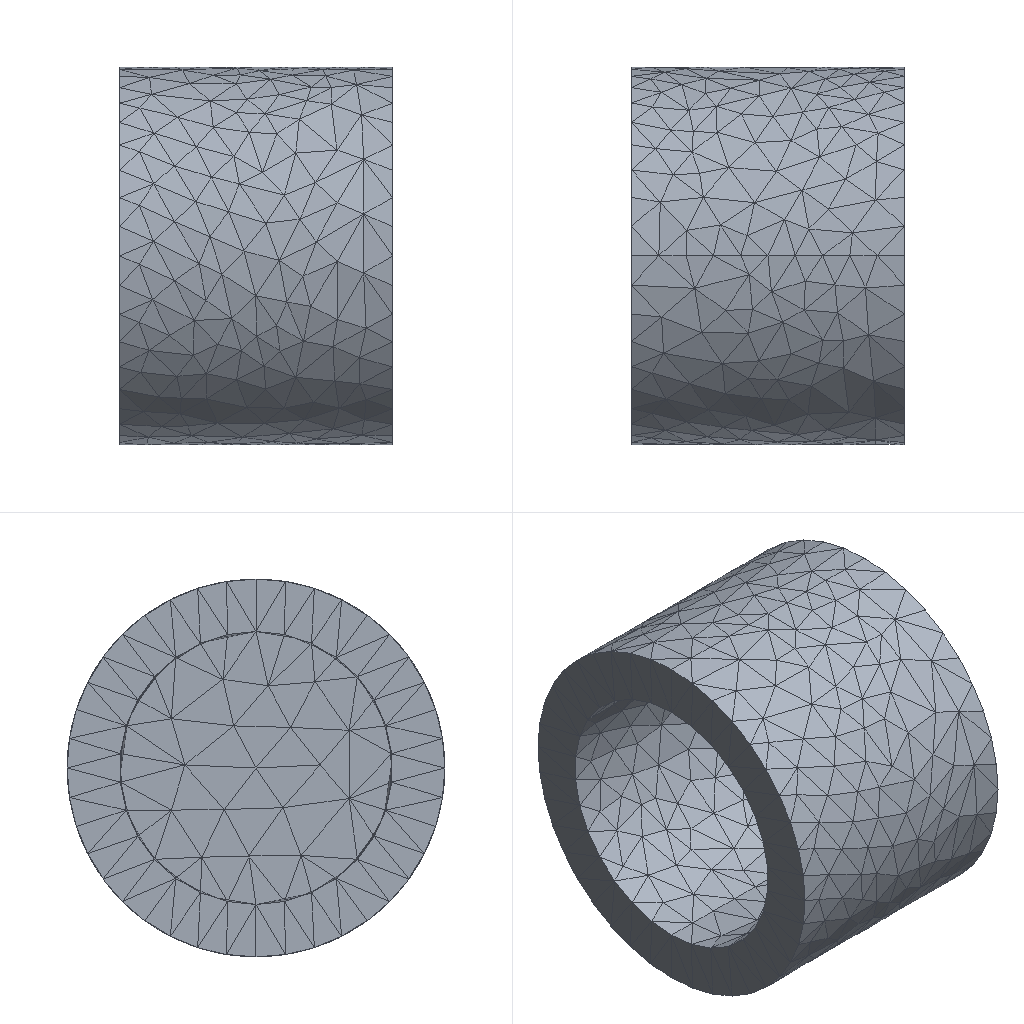Simulation study | ansys workbench
Ansys APDL input file, long lists of numbers shortened:
/batch
/config,noeldb,1     ! force off writing results to database
*get,_wallstrt,active,,time,wall
! ANSYS input file written by Workbench version 2022 R1
! File used for geometry attach:
/title,wbnew--____ (A5)
! ****** Begin Custom Load Command Snippet ******
/COM, ACT Extensions:
/COM,     LSDYNA, 2021.1
/COM,
! ****** End   Custom Load Command Snippet ******
*DIM,_wb_ProjectScratch_dir,string,248
_wb_ProjectScratch_dir(1) = ''
*DIM,_wb_SolverFiles_dir,string,248
_wb_SolverFiles_dir(1) = ''
*DIM,_wb_userfiles_dir,string,248
_wb_userfiles_dir(1) = ''
/com,--- Data in consistent NMM units. See Solving Units in the help system for more information.
/units,MPA
/nopr
/wb,file,start              !  signify a WB generated input file
/prep7
! Turn off shape checking because checks already performed inside WB mesher.
! See help system for more information.
SHPP,OFF,,NOWARN
/nolist
etcon,set             ! allow ANSYS to choose best KEYOP's for 180x elements, resets any applicable keyopt to MAPDL defaults
/com,*********** Nodes for the whole assembly ***********
nblock,3,,5248
(1i9,3e20.9e3)
        1     1.301000000E+03     0.000000000E+00     1.443258926E+02
! (4770 more lines like these left out)
-1
/wb,elem,start            !  set before creation of elements
/com,*********** Elements for Body 1 "__1-FreeParts|__-__6" ***********
et,1,187
eblock,19,solid,,2632
(19i9)
        1        1        1        1        0        0        0        0       10        0        1       12      767      445      696      833     3489      828      832
! (5263 more lines like these left out)
-1
/wb,elem,end               !  done creating elements
/com,*********** Send User Defined Coordinate System(s) ***********
csys,0
toffst,273.15,  ! Temperature offset from absolute zero
/com,*********** Set Reference Temperature ***********
tref,22.
/wb,mat,start              !  starting to send materials
/com,*********** Send Materials ***********
Temperature = 'TEMP' ! Temperature
MP,DENS,1,7.85e-09,	! tonne mm^-3
MP,ALPX,1,1.2e-05,	! C^-1
MP,C,1,434000000,	! mm^2 s^-2 C^-1
MP,KXX,1,60.5,	! tonne mm s^-3 C^-1
MP,RSVX,1,0.00017,	! ohm mm
MP,EX,1,200000,	! tonne s^-2 mm^-1
MP,NUXY,1,0.3,
MP,MURX,1,10000,
/wb,mat,end                !  done sending materials
!************************* Model Summary ********************
!__1-FreeParts|__-__6,	结构钢,	matid,	1
!************************* End Model Summary ********************
! get the diagonal of the bounding box. Needed later for other things
*get,_xmin,node,,mnloc,x
*get,_ymin,node,,mnloc,y
*get,_zmin,node,,mnloc,z
*get,_xmax,node,,mxloc,x
*get,_ymax,node,,mxloc,y
*get,_zmax,node,,mxloc,z
_ASMDIAG=(_xmax-_xmin)*(_xmax-_xmin)+(_ymax-_ymin)*(_ymax-_ymin)+(_zmax-_zmin)*(_zmax-_zmin)
_ASMDIAG=SQRT(_ASMDIAG)
/wb,contact,start          !  starting to send contact
/wb,contact,end            !  done creating contacts
/golist
/wb,load,start             !  starting to send loads
/com,*********** Fixed Supports ***********
CMBLOCK,_FIXEDSU,NODE,      245
(8i10)
         1         2         3         4         5         6         7         8
! (30 more lines like these left out)
cmsel,s,_FIXEDSU
d,all,all
nsel,all
/com,*********** Define Pressure Using Surface Effect Elements "__" ***********
et,2,154
eblock,10,,,622
(15i9)
     3845        2        2        2        0       23        2      152      152      775      776      152      891
! (621 more lines like these left out)
-1
esel,s,type,,2
keyop,2,7,0                ! Use deformed area for application of load
esel,all
/com,*********** Define Pressure Using Surface Effect Elements "__ 2" ***********
et,3,154
eblock,10,,,356
(15i9)
     4467        3        3        3        0      101      102      313      313     1458     1467      313     1460
! (355 more lines like these left out)
-1
esel,s,type,,3
keyop,3,7,0                ! Use deformed area for application of load
esel,all
esel,all
/gst,on,on
fini
*get,_numnode,node,0,count
*get,_numelem,elem,0,count
*get, _MAXELEMNUM, elem, 0, NUM, MAX
*get, _MAXNODENUM, node, 0, NUM, MAX
*get, _MAXELEMTYPE, etyp, 0, NUM, MAX
*get, _MAXREALCONST, real, 0, NUM, MAX
/go
/wb,load,end               !  done creating loads
/com,--- Number of total nodes = %_numnode%
/com,--- Number of contact elements = 978
/com,--- Number of spring elements = 0
/com,--- Number of bearing elements = 0
/com,--- Number of solid elements = 2632
/com,--- Number of condensed parts = 0
/com,--- Number of total elements = %_numelem%
*get,_wallbsol,active,,time,wall
/com,****************************************************************************
/com,*************************    SOLUTION       ********************************
/com,****************************************************************************
/solu
antype,0                   ! static analysis
_thickRatio=  0     ! Ratio of thick parts in the model
eqsl,sparse,,,,,1
cntr,print,1               ! print out contact info and also make no initial contact an error
dmpoption,emat,no             ! Don't combine emat file for DANSYS
dmpoption,esav,no             ! Don't combine esav file for DANSYS
nldiag,cont,iter           ! print out contact info each equilibrium iteration
rescontrol,,none                 ! Do not keep any restart files
/com,****************************************************
/com,******************* SOLVE FOR LS 1 OF 1 ****************
esel,s,type,,2
nsle
sf,all,pres,20.
esel,s,type,,3
nsle
sf,all,pres,60.
nsel,all
esel,all
esel,all
/nopr
/gopr
nsub,1,1,1
time,1.
outres,erase
outres,all,none
outres,nsol,all,
outres,rsol,all
outres,eangl,all
outres,etmp,all
outres,veng,all
outres,strs,all,
outres,epel,all,
outres,eppl,all,
outres,cont,all,
! *********** WB SOLVE COMMAND ***********
! check interactive state
*get,ANSINTER_,active,,int
*if,ANSINTER_,ne,0,then
/eof
*endif
solve
/com *************** Write FE CONNECTORS *********
CEWRITE,file,ce,,INTE
/com,****************************************************
/com,*************** FINISHED SOLVE FOR LS 1 *************
*get,_wallasol,active,,time,wall
/nopr
*get,_numnode,node,0,count
*get,_numelem,elem,0,count
*get, _MAXELEMNUM, elem, 0, NUM, MAX
*get, _MAXNODENUM, node, 0, NUM, MAX,,,INTERNAL
*get, _MAXELEMTYPE, etyp, 0, NUM, MAX
*get, _MAXREALCONST, real, 0, NUM, MAX
/gopr
/post1
xmlo,ENCODING,ISO-8859-1
xmlo,parm
/xml,parm,xml
fini
/gopr
*get,_walldone,active,,time,wall
_preptime=(_wallbsol-_wallstrt)*3600
_solvtime=(_wallasol-_wallbsol)*3600
_posttime=(_walldone-_wallasol)*3600
_totaltim=(_walldone-_wallstrt)*3600
*get,_dlbratio,active,0,solu,dlbr
*get,_combtime,active,0,solu,comb
*get,_ssmode,active,0,solu,ssmm
*get,_ndofs,active,0,solu,ndof
*get,_sol_end_time,active,0,set,time
*if,_sol_end_time,eq,1.,then
/fclean				!clean distributed files
*endif
/com,--- Total number of nodes = %_numnode%
/com,--- Total number of elements = %_numelem%
/com,--- Element load balance ratio = %_dlbratio%
/com,--- Time to combine distributed files = %_combtime%
/com,--- Sparse memory mode = %_ssmode%
/com,--- Number of DOF = %_ndofs%
/wb,file,end               ! done with WB generated input